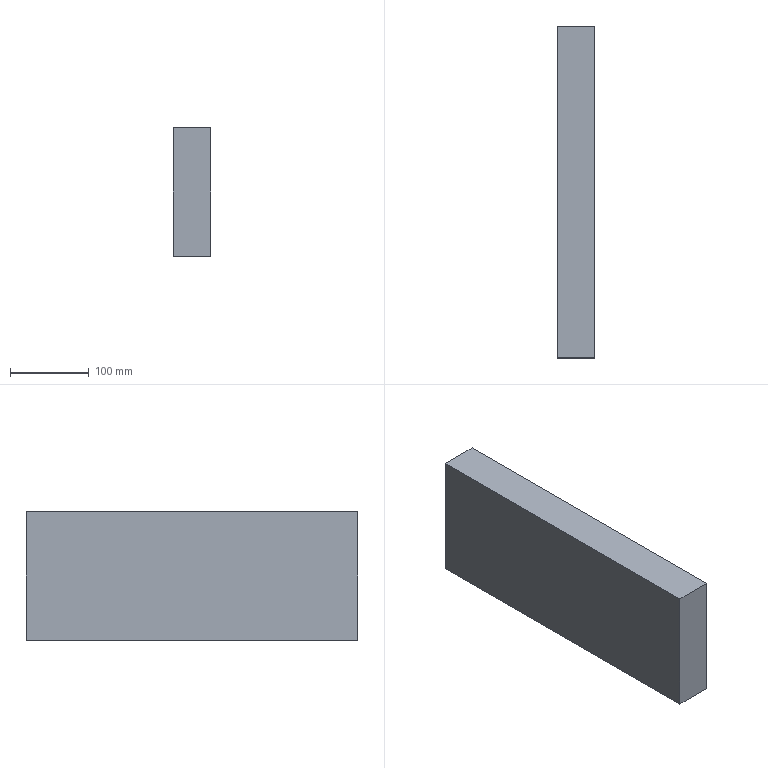Part | NX | features B2-5 2 | 1 solid | 12 faces | box 48 x 420 x 163 mm | volume 3270382 mm3 | plane 6 | cone 4 | cylinder 2 | commonest cylinder face diameters 14.506 x2
STEP:
#1=CARTESIAN_POINT('',(3792.094,-649.122,570.716));
#2=VERTEX_POINT('',#1);
#3=CARTESIAN_POINT('',(3840.094,-649.122,570.716));
#4=VERTEX_POINT('',#3);
#5=CARTESIAN_POINT('',(-540.,-649.122,570.716));
#6=DIRECTION('',(1.,0.,0.));
#7=VECTOR('',#6,1000.);
#8=LINE('',#5,#7);
#9=EDGE_CURVE('',#2,#4,#8,.T.);
#10=ORIENTED_EDGE('',*,*,#9,.F.);
#11=CARTESIAN_POINT('',(3792.094,-649.122,733.716));
#12=VERTEX_POINT('',#11);
#13=CARTESIAN_POINT('',(3792.094,-649.122,644.716));
#14=DIRECTION('',(0.,0.,-1.));
#15=VECTOR('',#14,1000.);
#16=LINE('',#13,#15);
#17=EDGE_CURVE('',#12,#2,#16,.T.);
#18=ORIENTED_EDGE('',*,*,#17,.F.);
#19=CARTESIAN_POINT('',(3840.094,-649.122,733.716));
#20=VERTEX_POINT('',#19);
#21=CARTESIAN_POINT('',(3816.094,-649.122,733.716));
#22=DIRECTION('',(-1.,0.,0.));
#23=VECTOR('',#22,1000.);
#24=LINE('',#21,#23);
#25=EDGE_CURVE('',#20,#12,#24,.T.);
#26=ORIENTED_EDGE('',*,*,#25,.F.);
#27=CARTESIAN_POINT('',(3840.094,-649.122,600.716));
#28=DIRECTION('',(0.,0.,-1.));
#29=VECTOR('',#28,1000.);
#30=LINE('',#27,#29);
#31=EDGE_CURVE('',#20,#4,#30,.T.);
#32=ORIENTED_EDGE('',*,*,#31,.T.);
#33=EDGE_LOOP('',(#10,#18,#26,#32));
#34=FACE_BOUND('',#33,.T.);
#35=CARTESIAN_POINT('',(3816.094,-649.122,644.716));
#36=DIRECTION('',(0.,1.,0.));
#37=DIRECTION('',(0.,0.,1.));
#38=AXIS2_PLACEMENT_3D('',#35,#36,#37);
#39=PLANE('',#38);
#40=ADVANCED_FACE('',(#34),#39,.T.);
#41=CARTESIAN_POINT('',(3792.094,-1069.122,570.716));
#42=VERTEX_POINT('',#41);
#43=CARTESIAN_POINT('',(3840.094,-1069.122,570.716));
#44=VERTEX_POINT('',#43);
#45=CARTESIAN_POINT('',(3816.094,-1069.122,570.716));
#46=DIRECTION('',(1.,0.,0.));
#47=VECTOR('',#46,1000.);
#48=LINE('',#45,#47);
#49=EDGE_CURVE('',#42,#44,#48,.T.);
#50=ORIENTED_EDGE('',*,*,#49,.T.);
#51=CARTESIAN_POINT('',(3840.094,-1069.122,733.716));
#52=VERTEX_POINT('',#51);
#53=CARTESIAN_POINT('',(3840.094,-1069.122,600.716));
#54=DIRECTION('',(0.,0.,1.));
#55=VECTOR('',#54,1000.);
#56=LINE('',#53,#55);
#57=EDGE_CURVE('',#44,#52,#56,.T.);
#58=ORIENTED_EDGE('',*,*,#57,.T.);
#59=CARTESIAN_POINT('',(3792.094,-1069.122,733.716));
#60=VERTEX_POINT('',#59);
#61=CARTESIAN_POINT('',(3816.094,-1069.122,733.716));
#62=DIRECTION('',(1.,0.,0.));
#63=VECTOR('',#62,1000.);
#64=LINE('',#61,#63);
#65=EDGE_CURVE('',#60,#52,#64,.T.);
#66=ORIENTED_EDGE('',*,*,#65,.F.);
#67=CARTESIAN_POINT('',(3792.094,-1069.122,644.716));
#68=DIRECTION('',(0.,0.,1.));
#69=VECTOR('',#68,1000.);
#70=LINE('',#67,#69);
#71=EDGE_CURVE('',#42,#60,#70,.T.);
#72=ORIENTED_EDGE('',*,*,#71,.F.);
#73=EDGE_LOOP('',(#50,#58,#66,#72));
#74=FACE_BOUND('',#73,.T.);
#75=CARTESIAN_POINT('',(3816.094,-1069.122,644.716));
#76=DIRECTION('',(0.,-1.,0.));
#77=DIRECTION('',(1.,0.,0.));
#78=AXIS2_PLACEMENT_3D('',#75,#76,#77);
#79=PLANE('',#78);
#80=ADVANCED_FACE('',(#74),#79,.T.);
#81=ORIENTED_EDGE('',*,*,#31,.F.);
#82=CARTESIAN_POINT('',(3840.094,-599.122,733.716));
#83=DIRECTION('',(0.,-1.,0.));
#84=VECTOR('',#83,1000.);
#85=LINE('',#82,#84);
#86=EDGE_CURVE('',#20,#52,#85,.T.);
#87=ORIENTED_EDGE('',*,*,#86,.T.);
#88=ORIENTED_EDGE('',*,*,#57,.F.);
#89=CARTESIAN_POINT('',(3840.094,-599.122,570.716));
#90=DIRECTION('',(0.,-1.,0.));
#91=VECTOR('',#90,1000.);
#92=LINE('',#89,#91);
#93=EDGE_CURVE('',#4,#44,#92,.T.);
#94=ORIENTED_EDGE('',*,*,#93,.F.);
#95=EDGE_LOOP('',(#81,#87,#88,#94));
#96=FACE_BOUND('',#95,.T.);
#97=CARTESIAN_POINT('',(3840.094,-599.122,600.716));
#98=DIRECTION('',(-1.,0.,0.));
#99=DIRECTION('',(0.,0.,1.));
#100=AXIS2_PLACEMENT_3D('',#97,#98,#99);
#101=PLANE('',#100);
#102=ADVANCED_FACE('',(#96),#101,.F.);
#103=CARTESIAN_POINT('',(3808.094,-669.122,570.716));
#104=VERTEX_POINT('',#103);
#105=CARTESIAN_POINT('',(3816.094,-669.122,570.716));
#106=DIRECTION('',(0.,0.,-1.));
#107=DIRECTION('',(-1.,0.,0.));
#108=AXIS2_PLACEMENT_3D('',#105,#106,#107);
#109=CIRCLE('',#108,8.);
#110=EDGE_CURVE('',#104,#104,#109,.T.);
#111=ORIENTED_EDGE('',*,*,#110,.F.);
#112=EDGE_LOOP('',(#111));
#113=FACE_BOUND('',#112,.T.);
#114=CARTESIAN_POINT('',(3808.094,-1049.122,570.716));
#115=VERTEX_POINT('',#114);
#116=CARTESIAN_POINT('',(3816.094,-1049.122,570.716));
#117=DIRECTION('',(0.,0.,-1.));
#118=DIRECTION('',(-1.,0.,0.));
#119=AXIS2_PLACEMENT_3D('',#116,#117,#118);
#120=CIRCLE('',#119,8.);
#121=EDGE_CURVE('',#115,#115,#120,.T.);
#122=ORIENTED_EDGE('',*,*,#121,.F.);
#123=EDGE_LOOP('',(#122));
#124=FACE_BOUND('',#123,.T.);
#125=CARTESIAN_POINT('',(3792.094,0.,570.716));
#126=DIRECTION('',(0.,-1.,0.));
#127=VECTOR('',#126,1000.);
#128=LINE('',#125,#127);
#129=EDGE_CURVE('',#2,#42,#128,.T.);
#130=ORIENTED_EDGE('',*,*,#129,.F.);
#131=ORIENTED_EDGE('',*,*,#9,.T.);
#132=ORIENTED_EDGE('',*,*,#93,.T.);
#133=ORIENTED_EDGE('',*,*,#49,.F.);
#134=EDGE_LOOP('',(#130,#131,#132,#133));
#135=FACE_BOUND('',#134,.T.);
#136=CARTESIAN_POINT('',(-540.,0.,570.716));
#137=DIRECTION('',(0.,0.,-1.));
#138=DIRECTION('',(-1.,0.,0.));
#139=AXIS2_PLACEMENT_3D('',#136,#137,#138);
#140=PLANE('',#139);
#141=ADVANCED_FACE('',(#113,#124,#135),#140,.T.);
#142=ORIENTED_EDGE('',*,*,#25,.T.);
#143=CARTESIAN_POINT('',(3792.094,-859.122,733.716));
#144=DIRECTION('',(0.,1.,0.));
#145=VECTOR('',#144,1000.);
#146=LINE('',#143,#145);
#147=EDGE_CURVE('',#60,#12,#146,.T.);
#148=ORIENTED_EDGE('',*,*,#147,.F.);
#149=ORIENTED_EDGE('',*,*,#65,.T.);
#150=ORIENTED_EDGE('',*,*,#86,.F.);
#151=EDGE_LOOP('',(#142,#148,#149,#150));
#152=FACE_BOUND('',#151,.T.);
#153=CARTESIAN_POINT('',(-540.,0.,733.716));
#154=DIRECTION('',(0.,0.,-1.));
#155=DIRECTION('',(-1.,0.,0.));
#156=AXIS2_PLACEMENT_3D('',#153,#154,#155);
#157=PLANE('',#156);
#158=ADVANCED_FACE('',(#152),#157,.F.);
#159=ORIENTED_EDGE('',*,*,#17,.T.);
#160=ORIENTED_EDGE('',*,*,#129,.T.);
#161=ORIENTED_EDGE('',*,*,#71,.T.);
#162=ORIENTED_EDGE('',*,*,#147,.T.);
#163=EDGE_LOOP('',(#159,#160,#161,#162));
#164=FACE_BOUND('',#163,.T.);
#165=CARTESIAN_POINT('',(3792.094,-859.122,667.216));
#166=DIRECTION('',(1.,0.,0.));
#167=DIRECTION('',(0.,0.,-1.));
#168=AXIS2_PLACEMENT_3D('',#165,#166,#167);
#169=PLANE('',#168);
#170=ADVANCED_FACE('',(#164),#169,.F.);
#171=CARTESIAN_POINT('',(3808.841,-1049.122,571.463));
#172=VERTEX_POINT('',#171);
#173=CARTESIAN_POINT('',(3816.094,-1049.122,571.463));
#174=DIRECTION('',(0.,0.,-1.));
#175=DIRECTION('',(-1.,0.,0.));
#176=AXIS2_PLACEMENT_3D('',#173,#174,#175);
#177=CIRCLE('',#176,7.253);
#178=EDGE_CURVE('',#172,#172,#177,.F.);
#179=ORIENTED_EDGE('',*,*,#178,.F.);
#180=EDGE_LOOP('',(#179));
#181=FACE_BOUND('',#180,.T.);
#182=CARTESIAN_POINT('',(3808.841,-1049.122,615.713));
#183=VERTEX_POINT('',#182);
#184=CARTESIAN_POINT('',(3816.094,-1049.122,615.713));
#185=DIRECTION('',(0.,0.,-1.));
#186=DIRECTION('',(-1.,0.,0.));
#187=AXIS2_PLACEMENT_3D('',#184,#185,#186);
#188=CIRCLE('',#187,7.253);
#189=EDGE_CURVE('',#183,#183,#188,.F.);
#190=ORIENTED_EDGE('',*,*,#189,.T.);
#191=EDGE_LOOP('',(#190));
#192=FACE_BOUND('',#191,.T.);
#193=CARTESIAN_POINT('',(3816.094,-1049.122,622.966));
#194=DIRECTION('',(0.,0.,-1.));
#195=DIRECTION('',(-1.,0.,0.));
#196=AXIS2_PLACEMENT_3D('',#193,#194,#195);
#197=CYLINDRICAL_SURFACE('',#196,7.253);
#198=ADVANCED_FACE('',(#181,#192),#197,.F.);
#199=CARTESIAN_POINT('',(3816.094,-1049.122,622.966));
#200=VERTEX_POINT('',#199);
#201=VERTEX_LOOP('',#200);
#202=FACE_BOUND('',#201,.T.);
#203=ORIENTED_EDGE('',*,*,#189,.F.);
#204=EDGE_LOOP('',(#203));
#205=FACE_BOUND('',#204,.T.);
#206=CARTESIAN_POINT('',(3816.094,-1049.122,615.716));
#207=DIRECTION('',(0.,0.,-1.));
#208=DIRECTION('',(-1.,0.,0.));
#209=AXIS2_PLACEMENT_3D('',#206,#207,#208);
#210=CONICAL_SURFACE('',#209,7.25,0.7854);
#211=ADVANCED_FACE('',(#202,#205),#210,.F.);
#212=ORIENTED_EDGE('',*,*,#178,.T.);
#213=EDGE_LOOP('',(#212));
#214=FACE_BOUND('',#213,.T.);
#215=ORIENTED_EDGE('',*,*,#121,.T.);
#216=EDGE_LOOP('',(#215));
#217=FACE_BOUND('',#216,.T.);
#218=CARTESIAN_POINT('',(3816.094,-1049.122,570.716));
#219=DIRECTION('',(0.,0.,-1.));
#220=DIRECTION('',(-1.,0.,0.));
#221=AXIS2_PLACEMENT_3D('',#218,#219,#220);
#222=CONICAL_SURFACE('',#221,8.,0.7854);
#223=ADVANCED_FACE('',(#214,#217),#222,.F.);
#224=CARTESIAN_POINT('',(3808.841,-669.122,571.463));
#225=VERTEX_POINT('',#224);
#226=CARTESIAN_POINT('',(3816.094,-669.122,571.463));
#227=DIRECTION('',(0.,0.,-1.));
#228=DIRECTION('',(-1.,0.,0.));
#229=AXIS2_PLACEMENT_3D('',#226,#227,#228);
#230=CIRCLE('',#229,7.253);
#231=EDGE_CURVE('',#225,#225,#230,.F.);
#232=ORIENTED_EDGE('',*,*,#231,.F.);
#233=EDGE_LOOP('',(#232));
#234=FACE_BOUND('',#233,.T.);
#235=CARTESIAN_POINT('',(3808.841,-669.122,615.713));
#236=VERTEX_POINT('',#235);
#237=CARTESIAN_POINT('',(3816.094,-669.122,615.713));
#238=DIRECTION('',(0.,0.,-1.));
#239=DIRECTION('',(-1.,0.,0.));
#240=AXIS2_PLACEMENT_3D('',#237,#238,#239);
#241=CIRCLE('',#240,7.253);
#242=EDGE_CURVE('',#236,#236,#241,.F.);
#243=ORIENTED_EDGE('',*,*,#242,.T.);
#244=EDGE_LOOP('',(#243));
#245=FACE_BOUND('',#244,.T.);
#246=CARTESIAN_POINT('',(3816.094,-669.122,622.966));
#247=DIRECTION('',(0.,0.,-1.));
#248=DIRECTION('',(-1.,0.,0.));
#249=AXIS2_PLACEMENT_3D('',#246,#247,#248);
#250=CYLINDRICAL_SURFACE('',#249,7.253);
#251=ADVANCED_FACE('',(#234,#245),#250,.F.);
#252=CARTESIAN_POINT('',(3816.094,-669.122,622.966));
#253=VERTEX_POINT('',#252);
#254=VERTEX_LOOP('',#253);
#255=FACE_BOUND('',#254,.T.);
#256=ORIENTED_EDGE('',*,*,#242,.F.);
#257=EDGE_LOOP('',(#256));
#258=FACE_BOUND('',#257,.T.);
#259=CARTESIAN_POINT('',(3816.094,-669.122,615.716));
#260=DIRECTION('',(0.,0.,-1.));
#261=DIRECTION('',(-1.,0.,0.));
#262=AXIS2_PLACEMENT_3D('',#259,#260,#261);
#263=CONICAL_SURFACE('',#262,7.25,0.7854);
#264=ADVANCED_FACE('',(#255,#258),#263,.F.);
#265=ORIENTED_EDGE('',*,*,#231,.T.);
#266=EDGE_LOOP('',(#265));
#267=FACE_BOUND('',#266,.T.);
#268=ORIENTED_EDGE('',*,*,#110,.T.);
#269=EDGE_LOOP('',(#268));
#270=FACE_BOUND('',#269,.T.);
#271=CARTESIAN_POINT('',(3816.094,-669.122,570.716));
#272=DIRECTION('',(0.,0.,-1.));
#273=DIRECTION('',(-1.,0.,0.));
#274=AXIS2_PLACEMENT_3D('',#271,#272,#273);
#275=CONICAL_SURFACE('',#274,8.,0.7854);
#276=ADVANCED_FACE('',(#267,#270),#275,.F.);
#277=CLOSED_SHELL('',(#40,#80,#102,#141,#158,#170,#198,#211,#223,#251,#264,#276));
#278=MANIFOLD_SOLID_BREP('',#277);
#279=(LENGTH_UNIT()NAMED_UNIT(*)SI_UNIT(.MILLI.,.METRE.));
#280=UNCERTAINTY_MEASURE_WITH_UNIT(LENGTH_MEASURE(0.00001),#279,'','');
#281=(NAMED_UNIT(*)PLANE_ANGLE_UNIT()SI_UNIT($,.RADIAN.));
#282=(NAMED_UNIT(*)SI_UNIT($,.STERADIAN.)SOLID_ANGLE_UNIT());
#283=(GEOMETRIC_REPRESENTATION_CONTEXT(3)GLOBAL_UNCERTAINTY_ASSIGNED_CONTEXT((#280))GLOBAL_UNIT_ASSIGNED_CONTEXT((#279,#281,#282))REPRESENTATION_CONTEXT('',''));
#284=ADVANCED_BREP_SHAPE_REPRESENTATION('',(#278),#283);